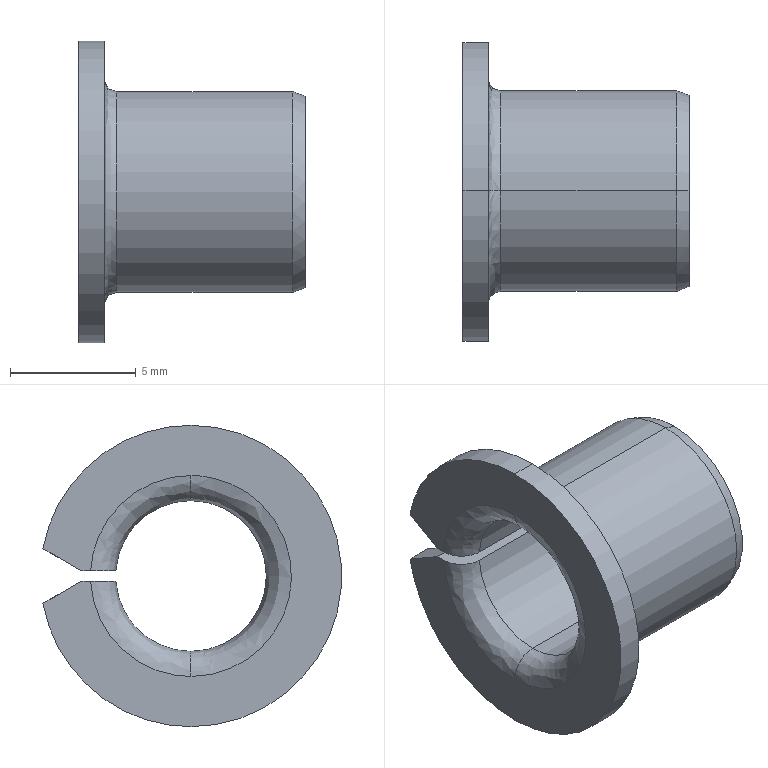Part | SolidWorks | features BaseBody 1 | 1 solid | 28 faces | box 9 x 11.899 x 12 mm | volume 248.45 mm3 | cylinder 9 | plane 7 | spline 6 | cone 6 | commonest cylinder face diameters 6 x3 8 x3 12 x3
STEP:
#1=CARTESIAN_POINT('',(1.5,0.,-4.));
#2=VERTEX_POINT('',#1);
#3=CARTESIAN_POINT('',(1.5,3.995,-0.2));
#4=VERTEX_POINT('',#3);
#5=CARTESIAN_POINT('',(1.5,0.,0.));
#6=DIRECTION('',(1.,0.,0.));
#7=DIRECTION('',(0.,0.,-1.));
#8=AXIS2_PLACEMENT_3D('',#5,#6,#7);
#9=CIRCLE('',#8,4.);
#10=EDGE_CURVE('',#2,#4,#9,.T.);
#11=ORIENTED_EDGE('',*,*,#10,.F.);
#12=CARTESIAN_POINT('',(1.,-0.000000039,-4.5));
#13=VERTEX_POINT('',#12);
#14=CARTESIAN_POINT('',(1.5,0.,-4.5));
#15=DIRECTION('',(0.,-1.,0.));
#16=DIRECTION('',(0.,0.,-1.));
#17=AXIS2_PLACEMENT_3D('',#14,#15,#16);
#18=CIRCLE('',#17,0.5);
#19=EDGE_CURVE('',#2,#13,#18,.T.);
#20=ORIENTED_EDGE('',*,*,#19,.T.);
#21=CARTESIAN_POINT('',(1.,4.491,-0.2835));
#22=VERTEX_POINT('',#21);
#23=CARTESIAN_POINT('',(1.,4.491,-0.2835));
#24=CARTESIAN_POINT('',(1.,4.456,-0.8322));
#25=CARTESIAN_POINT('',(1.,4.326,-1.356));
#26=CARTESIAN_POINT('',(1.,4.071,-1.919));
#27=CARTESIAN_POINT('',(1.,4.039,-1.986));
#28=CARTESIAN_POINT('',(1.,3.973,-2.115));
#29=CARTESIAN_POINT('',(1.,3.869,-2.306));
#30=CARTESIAN_POINT('',(1.,3.751,-2.49));
#31=CARTESIAN_POINT('',(1.,3.582,-2.727));
#32=CARTESIAN_POINT('',(1.,3.49,-2.845));
#33=CARTESIAN_POINT('',(1.,3.295,-3.068));
#34=CARTESIAN_POINT('',(1.,3.193,-3.175));
#35=CARTESIAN_POINT('',(1.,2.868,-3.48));
#36=CARTESIAN_POINT('',(1.,2.633,-3.661));
#37=CARTESIAN_POINT('',(1.,2.255,-3.897));
#38=CARTESIAN_POINT('',(1.,2.129,-3.967));
#39=CARTESIAN_POINT('',(1.,1.869,-4.096));
#40=CARTESIAN_POINT('',(1.,1.703,-4.169));
#41=CARTESIAN_POINT('',(1.,1.532,-4.231));
#42=CARTESIAN_POINT('',(1.,1.464,-4.256));
#43=CARTESIAN_POINT('',(1.,1.433,-4.266));
#44=CARTESIAN_POINT('',(1.,1.335,-4.298));
#45=CARTESIAN_POINT('',(1.,1.14,-4.357));
#46=CARTESIAN_POINT('',(1.,0.678,-4.464));
#47=CARTESIAN_POINT('',(1.,0.2735,-4.5));
#48=CARTESIAN_POINT('',(1.,-0.000000039,-4.5));
#49=B_SPLINE_CURVE_WITH_KNOTS('',3,(#23,#24,#25,#26,#27,#28,#29,#30,#31,#32,#33,#34,#35,#36,#37,#38,#39,#40,#41,#42,#43,#44,#45,#46,#47,#48),.UNSPECIFIED.,.F.,.F.,(4,2,2,1,2,2,2,2,2,1,2,2,1,1,4),(0.,0.06118,0.06883,0.07648,0.09177,0.1071,0.1224,0.153,0.1682,0.1835,0.1874,0.1912,0.1988,0.2141,0.2447),.UNSPECIFIED.);
#50=EDGE_CURVE('',#22,#13,#49,.T.);
#51=ORIENTED_EDGE('',*,*,#50,.F.);
#52=CARTESIAN_POINT('',(1.023,4.346,-0.2));
#53=VERTEX_POINT('',#52);
#54=CARTESIAN_POINT('',(1.,4.491,-0.2835));
#55=CARTESIAN_POINT('',(1.,4.442,-0.2552));
#56=CARTESIAN_POINT('',(1.008,4.394,-0.2273));
#57=CARTESIAN_POINT('',(1.023,4.346,-0.2));
#58=B_SPLINE_CURVE_WITH_KNOTS('',3,(#54,#55,#56,#57),.UNSPECIFIED.,.F.,.F.,(4,4),(0.,0.0001686),.UNSPECIFIED.);
#59=EDGE_CURVE('',#22,#53,#58,.T.);
#60=ORIENTED_EDGE('',*,*,#59,.T.);
#61=CARTESIAN_POINT('',(1.023,4.346,-0.2));
#62=CARTESIAN_POINT('',(1.054,4.245,-0.2));
#63=CARTESIAN_POINT('',(1.118,4.156,-0.2));
#64=CARTESIAN_POINT('',(1.289,4.03,-0.2));
#65=CARTESIAN_POINT('',(1.393,3.995,-0.2));
#66=CARTESIAN_POINT('',(1.5,3.995,-0.2));
#67=B_SPLINE_CURVE_WITH_KNOTS('',3,(#61,#62,#63,#64,#65,#66),.UNSPECIFIED.,.F.,.F.,(4,2,4),(0.,0.0003154,0.0006309),.UNSPECIFIED.);
#68=EDGE_CURVE('',#53,#4,#67,.T.);
#69=ORIENTED_EDGE('',*,*,#68,.T.);
#70=EDGE_LOOP('',(#11,#20,#51,#60,#69));
#71=FACE_OUTER_BOUND('',#70,.T.);
#72=CARTESIAN_POINT('',(1.5,3.997,-0.1473));
#73=CARTESIAN_POINT('',(1.5,3.913,-2.421));
#74=CARTESIAN_POINT('',(1.5,2.275,-4.));
#75=CARTESIAN_POINT('',(1.5,-0.000000035,-4.));
#76=CARTESIAN_POINT('',(1.207,3.997,-0.1473));
#77=CARTESIAN_POINT('',(1.207,3.913,-2.421));
#78=CARTESIAN_POINT('',(1.207,2.275,-4.));
#79=CARTESIAN_POINT('',(1.207,-0.000000035,-4.));
#80=CARTESIAN_POINT('',(1.,4.204,-0.1549));
#81=CARTESIAN_POINT('',(1.,4.116,-2.546));
#82=CARTESIAN_POINT('',(1.,2.393,-4.207));
#83=CARTESIAN_POINT('',(1.,-0.000000037,-4.207));
#84=CARTESIAN_POINT('',(1.,4.497,-0.1657));
#85=CARTESIAN_POINT('',(1.,4.403,-2.724));
#86=CARTESIAN_POINT('',(1.,2.56,-4.5));
#87=CARTESIAN_POINT('',(1.,-0.000000039,-4.5));
#88=(BOUNDED_SURFACE()B_SPLINE_SURFACE(3,3,((#72,#73,#74,#75),(#76,#77,#78,#79),(#80,#81,#82,#83),(#84,#85,#86,#87)),.UNSPECIFIED.,.F.,.F.,.F.)B_SPLINE_SURFACE_WITH_KNOTS((4,4),(4,4),(0.,1.),(0.,1.),.UNSPECIFIED.)GEOMETRIC_REPRESENTATION_ITEM()RATIONAL_B_SPLINE_SURFACE(((1.,0.8133,0.8133,1.),(0.8047,0.6545,0.6545,0.8047),(0.8047,0.6545,0.6545,0.8047),(1.,0.8133,0.8133,1.)))REPRESENTATION_ITEM('')SURFACE());
#89=ADVANCED_FACE('',(#71),#88,.F.);
#90=ORIENTED_EDGE('',*,*,#19,.F.);
#91=CARTESIAN_POINT('',(1.5,0.,4.));
#92=VERTEX_POINT('',#91);
#93=CARTESIAN_POINT('',(1.5,0.,0.));
#94=DIRECTION('',(1.,0.,0.));
#95=DIRECTION('',(0.,0.,-1.));
#96=AXIS2_PLACEMENT_3D('',#93,#94,#95);
#97=CIRCLE('',#96,4.);
#98=EDGE_CURVE('',#92,#2,#97,.T.);
#99=ORIENTED_EDGE('',*,*,#98,.F.);
#100=CARTESIAN_POINT('',(1.,-0.000000067,4.5));
#101=VERTEX_POINT('',#100);
#102=CARTESIAN_POINT('',(1.5,0.,4.5));
#103=DIRECTION('',(0.,1.,0.));
#104=DIRECTION('',(0.,0.,1.));
#105=AXIS2_PLACEMENT_3D('',#102,#103,#104);
#106=CIRCLE('',#105,0.5);
#107=EDGE_CURVE('',#92,#101,#106,.T.);
#108=ORIENTED_EDGE('',*,*,#107,.T.);
#109=CARTESIAN_POINT('',(1.,-0.000000039,-4.5));
#110=CARTESIAN_POINT('',(1.,-0.2853,-4.5));
#111=CARTESIAN_POINT('',(1.,-0.5701,-4.473));
#112=CARTESIAN_POINT('',(1.,-1.124,-4.367));
#113=CARTESIAN_POINT('',(1.,-1.395,-4.288));
#114=CARTESIAN_POINT('',(1.,-1.793,-4.13));
#115=CARTESIAN_POINT('',(1.,-1.934,-4.066));
#116=CARTESIAN_POINT('',(1.,-2.202,-3.927));
#117=CARTESIAN_POINT('',(1.,-2.333,-3.851));
#118=CARTESIAN_POINT('',(1.,-2.587,-3.685));
#119=CARTESIAN_POINT('',(1.,-2.713,-3.593));
#120=CARTESIAN_POINT('',(1.,-2.953,-3.399));
#121=CARTESIAN_POINT('',(1.,-3.068,-3.296));
#122=CARTESIAN_POINT('',(1.,-3.397,-2.967));
#123=CARTESIAN_POINT('',(1.,-3.592,-2.728));
#124=CARTESIAN_POINT('',(1.,-3.848,-2.339));
#125=CARTESIAN_POINT('',(1.,-3.923,-2.21));
#126=CARTESIAN_POINT('',(1.,-4.063,-1.941));
#127=CARTESIAN_POINT('',(1.,-4.125,-1.804));
#128=CARTESIAN_POINT('',(1.,-4.21,-1.592));
#129=CARTESIAN_POINT('',(1.,-4.234,-1.527));
#130=CARTESIAN_POINT('',(1.,-4.28,-1.392));
#131=CARTESIAN_POINT('',(1.,-4.345,-1.189));
#132=CARTESIAN_POINT('',(1.,-4.394,-0.9837));
#133=CARTESIAN_POINT('',(1.,-4.473,-0.5685));
#134=CARTESIAN_POINT('',(1.,-4.5,-0.2864));
#135=CARTESIAN_POINT('',(1.,-4.5,0.2866));
#136=CARTESIAN_POINT('',(1.,-4.46,0.709));
#137=CARTESIAN_POINT('',(1.,-4.345,1.189));
#138=CARTESIAN_POINT('',(1.,-4.28,1.392));
#139=CARTESIAN_POINT('',(1.,-4.234,1.527));
#140=CARTESIAN_POINT('',(1.,-4.21,1.592));
#141=CARTESIAN_POINT('',(1.,-4.126,1.803));
#142=CARTESIAN_POINT('',(1.,-4.063,1.941));
#143=CARTESIAN_POINT('',(1.,-3.923,2.209));
#144=CARTESIAN_POINT('',(1.,-3.847,2.339));
#145=CARTESIAN_POINT('',(1.,-3.593,2.727));
#146=CARTESIAN_POINT('',(1.,-3.397,2.968));
#147=CARTESIAN_POINT('',(1.,-3.068,3.295));
#148=CARTESIAN_POINT('',(1.,-2.954,3.399));
#149=CARTESIAN_POINT('',(1.,-2.714,3.593));
#150=CARTESIAN_POINT('',(1.,-2.587,3.685));
#151=CARTESIAN_POINT('',(1.,-2.333,3.851));
#152=CARTESIAN_POINT('',(1.,-2.203,3.927));
#153=CARTESIAN_POINT('',(1.,-1.934,4.066));
#154=CARTESIAN_POINT('',(1.,-1.793,4.13));
#155=CARTESIAN_POINT('',(1.,-1.395,4.288));
#156=CARTESIAN_POINT('',(1.,-1.124,4.367));
#157=CARTESIAN_POINT('',(1.,-0.5704,4.473));
#158=CARTESIAN_POINT('',(1.,-0.285,4.5));
#159=CARTESIAN_POINT('',(1.,-0.000000067,4.5));
#160=B_SPLINE_CURVE_WITH_KNOTS('',3,(#109,#110,#111,#112,#113,#114,#115,#116,#117,#118,#119,#120,#121,#122,#123,#124,#125,#126,#127,#128,#129,#130,#131,#132,#133,#134,#135,#136,#137,#138,#139,#140,#141,#142,#143,#144,#145,#146,#147,#148,#149,#150,#151,#152,#153,#154,#155,#156,#157,#158,#159),.UNSPECIFIED.,.F.,.F.,(4,2,2,2,2,2,2,2,2,2,2,1,2,2,1,1,2,2,2,2,2,2,2,2,2,2,4),(0.2447,0.2766,0.3085,0.3245,0.3405,0.3564,0.3724,0.4043,0.4202,0.4362,0.4442,0.4521,0.4681,0.5,0.5319,0.5479,0.5558,0.5638,0.5798,0.5957,0.6276,0.6436,0.6596,0.6755,0.6915,0.7234,0.7553),.UNSPECIFIED.);
#161=EDGE_CURVE('',#13,#101,#160,.T.);
#162=ORIENTED_EDGE('',*,*,#161,.F.);
#163=EDGE_LOOP('',(#90,#99,#108,#162));
#164=FACE_OUTER_BOUND('',#163,.T.);
#165=CARTESIAN_POINT('',(1.5,0.,-4.));
#166=CARTESIAN_POINT('',(1.5,-8.,-4.));
#167=CARTESIAN_POINT('',(1.5,-8.,4.));
#168=CARTESIAN_POINT('',(1.5,0.,4.));
#169=CARTESIAN_POINT('',(1.207,0.,-4.));
#170=CARTESIAN_POINT('',(1.207,-8.,-4.));
#171=CARTESIAN_POINT('',(1.207,-8.,4.));
#172=CARTESIAN_POINT('',(1.207,0.,4.));
#173=CARTESIAN_POINT('',(1.,0.,-4.207));
#174=CARTESIAN_POINT('',(1.,-8.414,-4.207));
#175=CARTESIAN_POINT('',(1.,-8.414,4.207));
#176=CARTESIAN_POINT('',(1.,0.,4.207));
#177=CARTESIAN_POINT('',(1.,0.,-4.5));
#178=CARTESIAN_POINT('',(1.,-9.,-4.5));
#179=CARTESIAN_POINT('',(1.,-9.,4.5));
#180=CARTESIAN_POINT('',(1.,0.,4.5));
#181=(BOUNDED_SURFACE()B_SPLINE_SURFACE(3,3,((#165,#166,#167,#168),(#169,#170,#171,#172),(#173,#174,#175,#176),(#177,#178,#179,#180)),.UNSPECIFIED.,.F.,.F.,.T.)B_SPLINE_SURFACE_WITH_KNOTS((4,4),(4,4),(0.,1.),(0.,1.),.UNSPECIFIED.)GEOMETRIC_REPRESENTATION_ITEM()RATIONAL_B_SPLINE_SURFACE(((1.,0.3333,0.3333,1.),(0.8047,0.2682,0.2682,0.8047),(0.8047,0.2682,0.2682,0.8047),(1.,0.3333,0.3333,1.)))REPRESENTATION_ITEM('')SURFACE());
#182=ADVANCED_FACE('',(#164),#181,.F.);
#183=CARTESIAN_POINT('',(1.,0.,3.));
#184=VERTEX_POINT('',#183);
#185=CARTESIAN_POINT('',(1.,0.,-3.));
#186=VERTEX_POINT('',#185);
#187=CARTESIAN_POINT('',(1.,0.,0.));
#188=DIRECTION('',(1.,0.,0.));
#189=DIRECTION('',(0.,0.,-1.));
#190=AXIS2_PLACEMENT_3D('',#187,#188,#189);
#191=CIRCLE('',#190,3.);
#192=EDGE_CURVE('',#184,#186,#191,.T.);
#193=ORIENTED_EDGE('',*,*,#192,.T.);
#194=CARTESIAN_POINT('',(0.,-0.000000037,-4.));
#195=VERTEX_POINT('',#194);
#196=CARTESIAN_POINT('',(1.,0.,-4.));
#197=DIRECTION('',(0.,-1.,0.));
#198=DIRECTION('',(0.,0.,-1.));
#199=AXIS2_PLACEMENT_3D('',#196,#197,#198);
#200=CIRCLE('',#199,1.);
#201=EDGE_CURVE('',#186,#195,#200,.T.);
#202=ORIENTED_EDGE('',*,*,#201,.T.);
#203=CARTESIAN_POINT('',(0.,-0.000000017,4.));
#204=VERTEX_POINT('',#203);
#205=CARTESIAN_POINT('',(0.,-0.000000037,-4.));
#206=CARTESIAN_POINT('',(0.,-8.,-4.));
#207=CARTESIAN_POINT('',(0.,-8.,4.));
#208=CARTESIAN_POINT('',(0.,-0.000000017,4.));
#209=(BOUNDED_CURVE()B_SPLINE_CURVE(3,(#205,#206,#207,#208),.UNSPECIFIED.,.F.,.F.)B_SPLINE_CURVE_WITH_KNOTS((4,4),(0.246,0.754),.UNSPECIFIED.)CURVE()GEOMETRIC_REPRESENTATION_ITEM()RATIONAL_B_SPLINE_CURVE((1.,0.3333,0.3333,1.))REPRESENTATION_ITEM(''));
#210=EDGE_CURVE('',#195,#204,#209,.T.);
#211=ORIENTED_EDGE('',*,*,#210,.T.);
#212=CARTESIAN_POINT('',(1.,0.,4.));
#213=DIRECTION('',(0.,1.,0.));
#214=DIRECTION('',(0.,0.,1.));
#215=AXIS2_PLACEMENT_3D('',#212,#213,#214);
#216=CIRCLE('',#215,1.);
#217=EDGE_CURVE('',#184,#204,#216,.T.);
#218=ORIENTED_EDGE('',*,*,#217,.F.);
#219=EDGE_LOOP('',(#193,#202,#211,#218));
#220=FACE_OUTER_BOUND('',#219,.T.);
#221=CARTESIAN_POINT('',(1.,0.,-3.));
#222=CARTESIAN_POINT('',(1.,-6.,-3.));
#223=CARTESIAN_POINT('',(1.,-6.,3.));
#224=CARTESIAN_POINT('',(1.,0.,3.));
#225=CARTESIAN_POINT('',(0.4142,0.,-3.));
#226=CARTESIAN_POINT('',(0.4142,-6.,-3.));
#227=CARTESIAN_POINT('',(0.4142,-6.,3.));
#228=CARTESIAN_POINT('',(0.4142,0.,3.));
#229=CARTESIAN_POINT('',(0.,0.,-3.414));
#230=CARTESIAN_POINT('',(0.,-6.828,-3.414));
#231=CARTESIAN_POINT('',(0.,-6.828,3.414));
#232=CARTESIAN_POINT('',(0.,0.,3.414));
#233=CARTESIAN_POINT('',(0.,0.,-4.));
#234=CARTESIAN_POINT('',(0.,-8.,-4.));
#235=CARTESIAN_POINT('',(0.,-8.,4.));
#236=CARTESIAN_POINT('',(0.,0.,4.));
#237=(BOUNDED_SURFACE()B_SPLINE_SURFACE(3,3,((#221,#222,#223,#224),(#225,#226,#227,#228),(#229,#230,#231,#232),(#233,#234,#235,#236)),.UNSPECIFIED.,.F.,.F.,.T.)B_SPLINE_SURFACE_WITH_KNOTS((4,4),(4,4),(0.,1.),(0.,1.),.UNSPECIFIED.)GEOMETRIC_REPRESENTATION_ITEM()RATIONAL_B_SPLINE_SURFACE(((1.,0.3333,0.3333,1.),(0.8047,0.2682,0.2682,0.8047),(0.8047,0.2682,0.2682,0.8047),(1.,0.3333,0.3333,1.)))REPRESENTATION_ITEM('')SURFACE());
#238=ADVANCED_FACE('',(#220),#237,.T.);
#239=CARTESIAN_POINT('',(1.,2.993,0.2));
#240=VERTEX_POINT('',#239);
#241=CARTESIAN_POINT('',(1.,0.,0.));
#242=DIRECTION('',(1.,0.,0.));
#243=DIRECTION('',(0.,0.,-1.));
#244=AXIS2_PLACEMENT_3D('',#241,#242,#243);
#245=CIRCLE('',#244,3.);
#246=EDGE_CURVE('',#240,#184,#245,.T.);
#247=ORIENTED_EDGE('',*,*,#246,.T.);
#248=ORIENTED_EDGE('',*,*,#217,.T.);
#249=CARTESIAN_POINT('',(0.,3.995,0.2));
#250=VERTEX_POINT('',#249);
#251=CARTESIAN_POINT('',(0.,-0.000000017,4.));
#252=CARTESIAN_POINT('',(0.,2.251,4.));
#253=CARTESIAN_POINT('',(0.,3.882,2.448));
#254=CARTESIAN_POINT('',(0.,3.995,0.2));
#255=(BOUNDED_CURVE()B_SPLINE_CURVE(3,(#251,#252,#253,#254),.UNSPECIFIED.,.F.,.F.)B_SPLINE_CURVE_WITH_KNOTS((4,4),(0.754,1.),.UNSPECIFIED.)CURVE()GEOMETRIC_REPRESENTATION_ITEM()RATIONAL_B_SPLINE_CURVE((1.,0.8164,0.8164,1.))REPRESENTATION_ITEM(''));
#256=EDGE_CURVE('',#204,#250,#255,.T.);
#257=ORIENTED_EDGE('',*,*,#256,.T.);
#258=CARTESIAN_POINT('',(0.,3.995,0.2));
#259=CARTESIAN_POINT('',(0.,3.863,0.2));
#260=CARTESIAN_POINT('',(0.02595,3.733,0.2));
#261=CARTESIAN_POINT('',(0.1261,3.491,0.2));
#262=CARTESIAN_POINT('',(0.2003,3.38,0.2));
#263=CARTESIAN_POINT('',(0.4767,3.102,0.2));
#264=CARTESIAN_POINT('',(0.7357,2.993,0.2));
#265=CARTESIAN_POINT('',(1.,2.993,0.2));
#266=B_SPLINE_CURVE_WITH_KNOTS('',3,(#258,#259,#260,#261,#262,#263,#264,#265),.UNSPECIFIED.,.F.,.F.,(4,2,2,4),(0.,0.0003909,0.0007817,0.001563),.UNSPECIFIED.);
#267=EDGE_CURVE('',#250,#240,#266,.T.);
#268=ORIENTED_EDGE('',*,*,#267,.T.);
#269=EDGE_LOOP('',(#247,#248,#257,#268));
#270=FACE_OUTER_BOUND('',#269,.T.);
#271=CARTESIAN_POINT('',(1.,-0.000000006,3.));
#272=CARTESIAN_POINT('',(1.,1.701,3.));
#273=CARTESIAN_POINT('',(1.,2.928,1.822));
#274=CARTESIAN_POINT('',(1.,2.997,0.1227));
#275=CARTESIAN_POINT('',(0.4142,-0.000000006,3.));
#276=CARTESIAN_POINT('',(0.4142,1.701,3.));
#277=CARTESIAN_POINT('',(0.4142,2.928,1.822));
#278=CARTESIAN_POINT('',(0.4142,2.997,0.1227));
#279=CARTESIAN_POINT('',(0.,-0.000000007,3.414));
#280=CARTESIAN_POINT('',(0.,1.936,3.414));
#281=CARTESIAN_POINT('',(0.,3.332,2.074));
#282=CARTESIAN_POINT('',(0.,3.411,0.1396));
#283=CARTESIAN_POINT('',(0.,-0.000000008,4.));
#284=CARTESIAN_POINT('',(0.,2.268,4.));
#285=CARTESIAN_POINT('',(0.,3.904,2.43));
#286=CARTESIAN_POINT('',(0.,3.997,0.1635));
#287=(BOUNDED_SURFACE()B_SPLINE_SURFACE(3,3,((#271,#272,#273,#274),(#275,#276,#277,#278),(#279,#280,#281,#282),(#283,#284,#285,#286)),.UNSPECIFIED.,.F.,.F.,.F.)B_SPLINE_SURFACE_WITH_KNOTS((4,4),(4,4),(0.,1.),(0.,1.),.UNSPECIFIED.)GEOMETRIC_REPRESENTATION_ITEM()RATIONAL_B_SPLINE_SURFACE(((1.,0.8143,0.8143,1.),(0.8047,0.6553,0.6553,0.8047),(0.8047,0.6553,0.6553,0.8047),(1.,0.8143,0.8143,1.)))REPRESENTATION_ITEM('')SURFACE());
#288=ADVANCED_FACE('',(#270),#287,.T.);
#289=CARTESIAN_POINT('',(1.5,3.995,0.2));
#290=VERTEX_POINT('',#289);
#291=CARTESIAN_POINT('',(1.5,0.,0.));
#292=DIRECTION('',(1.,0.,0.));
#293=DIRECTION('',(0.,0.,-1.));
#294=AXIS2_PLACEMENT_3D('',#291,#292,#293);
#295=CIRCLE('',#294,4.);
#296=EDGE_CURVE('',#290,#92,#295,.T.);
#297=ORIENTED_EDGE('',*,*,#296,.T.);
#298=CARTESIAN_POINT('',(8.5,0.,4.));
#299=VERTEX_POINT('',#298);
#300=CARTESIAN_POINT('',(5.,0.,4.));
#301=DIRECTION('',(1.,0.,0.));
#302=VECTOR('',#301,1000.);
#303=LINE('',#300,#302);
#304=EDGE_CURVE('',#92,#299,#303,.T.);
#305=ORIENTED_EDGE('',*,*,#304,.T.);
#306=CARTESIAN_POINT('',(8.5,3.995,0.2));
#307=VERTEX_POINT('',#306);
#308=CARTESIAN_POINT('',(8.5,0.,0.));
#309=DIRECTION('',(-1.,0.,0.));
#310=DIRECTION('',(0.,0.,-1.));
#311=AXIS2_PLACEMENT_3D('',#308,#309,#310);
#312=CIRCLE('',#311,4.);
#313=EDGE_CURVE('',#299,#307,#312,.T.);
#314=ORIENTED_EDGE('',*,*,#313,.T.);
#315=CARTESIAN_POINT('',(5.,3.995,0.2));
#316=DIRECTION('',(-1.,0.,0.));
#317=VECTOR('',#316,1000.);
#318=LINE('',#315,#317);
#319=EDGE_CURVE('',#307,#290,#318,.T.);
#320=ORIENTED_EDGE('',*,*,#319,.T.);
#321=EDGE_LOOP('',(#297,#305,#314,#320));
#322=FACE_OUTER_BOUND('',#321,.T.);
#323=CARTESIAN_POINT('',(5.,0.,0.));
#324=DIRECTION('',(1.,0.,0.));
#325=DIRECTION('',(0.,0.,-1.));
#326=AXIS2_PLACEMENT_3D('',#323,#324,#325);
#327=CYLINDRICAL_SURFACE('',#326,4.);
#328=ADVANCED_FACE('',(#322),#327,.T.);
#329=ORIENTED_EDGE('',*,*,#304,.F.);
#330=ORIENTED_EDGE('',*,*,#98,.T.);
#331=CARTESIAN_POINT('',(8.5,0.,-4.));
#332=VERTEX_POINT('',#331);
#333=CARTESIAN_POINT('',(5.,0.,-4.));
#334=DIRECTION('',(1.,0.,0.));
#335=VECTOR('',#334,1000.);
#336=LINE('',#333,#335);
#337=EDGE_CURVE('',#2,#332,#336,.T.);
#338=ORIENTED_EDGE('',*,*,#337,.T.);
#339=CARTESIAN_POINT('',(8.5,0.,0.));
#340=DIRECTION('',(-1.,0.,0.));
#341=DIRECTION('',(0.,0.,-1.));
#342=AXIS2_PLACEMENT_3D('',#339,#340,#341);
#343=CIRCLE('',#342,4.);
#344=EDGE_CURVE('',#332,#299,#343,.T.);
#345=ORIENTED_EDGE('',*,*,#344,.T.);
#346=EDGE_LOOP('',(#329,#330,#338,#345));
#347=FACE_OUTER_BOUND('',#346,.T.);
#348=CARTESIAN_POINT('',(5.,0.,0.));
#349=DIRECTION('',(1.,0.,0.));
#350=DIRECTION('',(0.,0.,-1.));
#351=AXIS2_PLACEMENT_3D('',#348,#349,#350);
#352=CYLINDRICAL_SURFACE('',#351,4.);
#353=ADVANCED_FACE('',(#347),#352,.T.);
#354=CARTESIAN_POINT('',(9.,3.813,-0.2));
#355=VERTEX_POINT('',#354);
#356=CARTESIAN_POINT('',(9.,0.,-3.818));
#357=VERTEX_POINT('',#356);
#358=CARTESIAN_POINT('',(9.,0.,0.));
#359=DIRECTION('',(-1.,0.,0.));
#360=DIRECTION('',(0.,0.,1.));
#361=AXIS2_PLACEMENT_3D('',#358,#359,#360);
#362=CIRCLE('',#361,3.818);
#363=EDGE_CURVE('',#355,#357,#362,.T.);
#364=ORIENTED_EDGE('',*,*,#363,.T.);
#365=CARTESIAN_POINT('',(8.5,0.,-4.));
#366=DIRECTION('',(-0.9397,0.,-0.342));
#367=VECTOR('',#366,1000.);
#368=LINE('',#365,#367);
#369=EDGE_CURVE('',#357,#332,#368,.T.);
#370=ORIENTED_EDGE('',*,*,#369,.T.);
#371=CARTESIAN_POINT('',(8.5,3.995,-0.2));
#372=VERTEX_POINT('',#371);
#373=CARTESIAN_POINT('',(8.5,0.,0.));
#374=DIRECTION('',(-1.,0.,0.));
#375=DIRECTION('',(0.,0.,-1.));
#376=AXIS2_PLACEMENT_3D('',#373,#374,#375);
#377=CIRCLE('',#376,4.);
#378=EDGE_CURVE('',#372,#332,#377,.T.);
#379=ORIENTED_EDGE('',*,*,#378,.F.);
#380=CARTESIAN_POINT('',(8.5,3.995,-0.2));
#381=CARTESIAN_POINT('',(8.667,3.934,-0.2));
#382=CARTESIAN_POINT('',(8.833,3.874,-0.2));
#383=CARTESIAN_POINT('',(9.,3.813,-0.2));
#384=B_SPLINE_CURVE_WITH_KNOTS('',3,(#380,#381,#382,#383),.UNSPECIFIED.,.F.,.F.,(4,4),(0.,0.0005322),.UNSPECIFIED.);
#385=EDGE_CURVE('',#372,#355,#384,.T.);
#386=ORIENTED_EDGE('',*,*,#385,.T.);
#387=EDGE_LOOP('',(#364,#370,#379,#386));
#388=FACE_OUTER_BOUND('',#387,.T.);
#389=CARTESIAN_POINT('',(8.5,0.,0.));
#390=DIRECTION('',(-1.,0.,0.));
#391=DIRECTION('',(0.,0.,1.));
#392=AXIS2_PLACEMENT_3D('',#389,#390,#391);
#393=CONICAL_SURFACE('',#392,4.,0.3491);
#394=ADVANCED_FACE('',(#388),#393,.T.);
#395=ORIENTED_EDGE('',*,*,#369,.F.);
#396=CARTESIAN_POINT('',(9.,0.,3.818));
#397=VERTEX_POINT('',#396);
#398=CARTESIAN_POINT('',(9.,0.,0.));
#399=DIRECTION('',(-1.,0.,0.));
#400=DIRECTION('',(0.,0.,1.));
#401=AXIS2_PLACEMENT_3D('',#398,#399,#400);
#402=CIRCLE('',#401,3.818);
#403=EDGE_CURVE('',#357,#397,#402,.T.);
#404=ORIENTED_EDGE('',*,*,#403,.T.);
#405=CARTESIAN_POINT('',(8.5,0.,4.));
#406=DIRECTION('',(-0.9397,0.,0.342));
#407=VECTOR('',#406,1000.);
#408=LINE('',#405,#407);
#409=EDGE_CURVE('',#397,#299,#408,.T.);
#410=ORIENTED_EDGE('',*,*,#409,.T.);
#411=ORIENTED_EDGE('',*,*,#344,.F.);
#412=EDGE_LOOP('',(#395,#404,#410,#411));
#413=FACE_OUTER_BOUND('',#412,.T.);
#414=CARTESIAN_POINT('',(8.5,0.,0.));
#415=DIRECTION('',(-1.,0.,0.));
#416=DIRECTION('',(0.,0.,1.));
#417=AXIS2_PLACEMENT_3D('',#414,#415,#416);
#418=CONICAL_SURFACE('',#417,4.,0.3491);
#419=ADVANCED_FACE('',(#413),#418,.T.);
#420=ORIENTED_EDGE('',*,*,#192,.F.);
#421=CARTESIAN_POINT('',(8.5,0.,3.));
#422=VERTEX_POINT('',#421);
#423=CARTESIAN_POINT('',(4.75,0.,3.));
#424=DIRECTION('',(1.,0.,0.));
#425=VECTOR('',#424,1000.);
#426=LINE('',#423,#425);
#427=EDGE_CURVE('',#184,#422,#426,.T.);
#428=ORIENTED_EDGE('',*,*,#427,.T.);
#429=CARTESIAN_POINT('',(8.5,0.,-3.));
#430=VERTEX_POINT('',#429);
#431=CARTESIAN_POINT('',(8.5,0.,0.));
#432=DIRECTION('',(-1.,0.,0.));
#433=DIRECTION('',(0.,0.,-1.));
#434=AXIS2_PLACEMENT_3D('',#431,#432,#433);
#435=CIRCLE('',#434,3.);
#436=EDGE_CURVE('',#430,#422,#435,.T.);
#437=ORIENTED_EDGE('',*,*,#436,.F.);
#438=CARTESIAN_POINT('',(4.75,0.,-3.));
#439=DIRECTION('',(1.,0.,0.));
#440=VECTOR('',#439,1000.);
#441=LINE('',#438,#440);
#442=EDGE_CURVE('',#186,#430,#441,.T.);
#443=ORIENTED_EDGE('',*,*,#442,.F.);
#444=EDGE_LOOP('',(#420,#428,#437,#443));
#445=FACE_OUTER_BOUND('',#444,.T.);
#446=CARTESIAN_POINT('',(4.75,0.,0.));
#447=DIRECTION('',(1.,0.,0.));
#448=DIRECTION('',(0.,0.,-1.));
#449=AXIS2_PLACEMENT_3D('',#446,#447,#448);
#450=CYLINDRICAL_SURFACE('',#449,3.);
#451=ADVANCED_FACE('',(#445),#450,.F.);
#452=CARTESIAN_POINT('',(1.,2.993,-0.2));
#453=VERTEX_POINT('',#452);
#454=CARTESIAN_POINT('',(1.,0.,0.));
#455=DIRECTION('',(1.,0.,0.));
#456=DIRECTION('',(0.,0.,-1.));
#457=AXIS2_PLACEMENT_3D('',#454,#455,#456);
#458=CIRCLE('',#457,3.);
#459=EDGE_CURVE('',#186,#453,#458,.T.);
#460=ORIENTED_EDGE('',*,*,#459,.F.);
#461=ORIENTED_EDGE('',*,*,#442,.T.);
#462=CARTESIAN_POINT('',(8.5,2.993,-0.2));
#463=VERTEX_POINT('',#462);
#464=CARTESIAN_POINT('',(8.5,0.,0.));
#465=DIRECTION('',(-1.,0.,0.));
#466=DIRECTION('',(0.,0.,-1.));
#467=AXIS2_PLACEMENT_3D('',#464,#465,#466);
#468=CIRCLE('',#467,3.);
#469=EDGE_CURVE('',#463,#430,#468,.T.);
#470=ORIENTED_EDGE('',*,*,#469,.F.);
#471=CARTESIAN_POINT('',(0.,2.993,-0.2));
#472=DIRECTION('',(-1.,0.,0.));
#473=VECTOR('',#472,1000.);
#474=LINE('',#471,#473);
#475=EDGE_CURVE('',#463,#453,#474,.T.);
#476=ORIENTED_EDGE('',*,*,#475,.T.);
#477=EDGE_LOOP('',(#460,#461,#470,#476));
#478=FACE_OUTER_BOUND('',#477,.T.);
#479=CARTESIAN_POINT('',(4.75,0.,0.));
#480=DIRECTION('',(1.,0.,0.));
#481=DIRECTION('',(0.,0.,-1.));
#482=AXIS2_PLACEMENT_3D('',#479,#480,#481);
#483=CYLINDRICAL_SURFACE('',#482,3.);
#484=ADVANCED_FACE('',(#478),#483,.F.);
#485=ORIENTED_EDGE('',*,*,#436,.T.);
#486=CARTESIAN_POINT('',(9.,0.,3.5));
#487=VERTEX_POINT('',#486);
#488=CARTESIAN_POINT('',(9.,0.,3.5));
#489=DIRECTION('',(0.7071,0.,0.7071));
#490=VECTOR('',#489,1000.);
#491=LINE('',#488,#490);
#492=EDGE_CURVE('',#422,#487,#491,.T.);
#493=ORIENTED_EDGE('',*,*,#492,.T.);
#494=CARTESIAN_POINT('',(9.,0.,-3.5));
#495=VERTEX_POINT('',#494);
#496=CARTESIAN_POINT('',(9.,0.,0.));
#497=DIRECTION('',(-1.,0.,0.));
#498=DIRECTION('',(0.,0.,-1.));
#499=AXIS2_PLACEMENT_3D('',#496,#497,#498);
#500=CIRCLE('',#499,3.5);
#501=EDGE_CURVE('',#495,#487,#500,.T.);
#502=ORIENTED_EDGE('',*,*,#501,.F.);
#503=CARTESIAN_POINT('',(9.,0.,-3.5));
#504=DIRECTION('',(0.7071,0.,-0.7071));
#505=VECTOR('',#504,1000.);
#506=LINE('',#503,#505);
#507=EDGE_CURVE('',#430,#495,#506,.T.);
#508=ORIENTED_EDGE('',*,*,#507,.F.);
#509=EDGE_LOOP('',(#485,#493,#502,#508));
#510=FACE_OUTER_BOUND('',#509,.T.);
#511=CARTESIAN_POINT('',(9.,0.,0.));
#512=DIRECTION('',(1.,0.,0.));
#513=DIRECTION('',(0.,0.,-1.));
#514=AXIS2_PLACEMENT_3D('',#511,#512,#513);
#515=CONICAL_SURFACE('',#514,3.5,0.7854);
#516=ADVANCED_FACE('',(#510),#515,.F.);
#517=ORIENTED_EDGE('',*,*,#469,.T.);
#518=ORIENTED_EDGE('',*,*,#507,.T.);
#519=CARTESIAN_POINT('',(9.,3.494,-0.2));
#520=VERTEX_POINT('',#519);
#521=CARTESIAN_POINT('',(9.,0.,0.));
#522=DIRECTION('',(-1.,0.,0.));
#523=DIRECTION('',(0.,0.,-1.));
#524=AXIS2_PLACEMENT_3D('',#521,#522,#523);
#525=CIRCLE('',#524,3.5);
#526=EDGE_CURVE('',#520,#495,#525,.T.);
#527=ORIENTED_EDGE('',*,*,#526,.F.);
#528=CARTESIAN_POINT('',(8.5,2.993,-0.2));
#529=CARTESIAN_POINT('',(8.667,3.16,-0.2));
#530=CARTESIAN_POINT('',(8.833,3.327,-0.2));
#531=CARTESIAN_POINT('',(9.,3.494,-0.2));
#532=B_SPLINE_CURVE_WITH_KNOTS('',3,(#528,#529,#530,#531),.UNSPECIFIED.,.F.,.F.,(4,4),(0.,0.0007078),.UNSPECIFIED.);
#533=EDGE_CURVE('',#463,#520,#532,.T.);
#534=ORIENTED_EDGE('',*,*,#533,.F.);
#535=EDGE_LOOP('',(#517,#518,#527,#534));
#536=FACE_OUTER_BOUND('',#535,.T.);
#537=CARTESIAN_POINT('',(9.,0.,0.));
#538=DIRECTION('',(1.,0.,0.));
#539=DIRECTION('',(0.,0.,-1.));
#540=AXIS2_PLACEMENT_3D('',#537,#538,#539);
#541=CONICAL_SURFACE('',#540,3.5,0.7854);
#542=ADVANCED_FACE('',(#536),#541,.F.);
#543=CARTESIAN_POINT('',(0.,0.,6.));
#544=VERTEX_POINT('',#543);
#545=CARTESIAN_POINT('',(0.,5.899,1.096));
#546=VERTEX_POINT('',#545);
#547=CARTESIAN_POINT('',(0.,0.,0.));
#548=DIRECTION('',(-1.,0.,0.));
#549=DIRECTION('',(0.,0.,-1.));
#550=AXIS2_PLACEMENT_3D('',#547,#548,#549);
#551=CIRCLE('',#550,6.);
#552=EDGE_CURVE('',#544,#546,#551,.T.);
#553=ORIENTED_EDGE('',*,*,#552,.F.);
#554=CARTESIAN_POINT('',(1.,0.,6.));
#555=VERTEX_POINT('',#554);
#556=CARTESIAN_POINT('',(0.5,0.,6.));
#557=DIRECTION('',(1.,0.,0.));
#558=VECTOR('',#557,1000.);
#559=LINE('',#556,#558);
#560=EDGE_CURVE('',#544,#555,#559,.T.);
#561=ORIENTED_EDGE('',*,*,#560,.T.);
#562=CARTESIAN_POINT('',(1.,5.899,1.096));
#563=VERTEX_POINT('',#562);
#564=CARTESIAN_POINT('',(1.,0.,0.));
#565=DIRECTION('',(1.,0.,0.));
#566=DIRECTION('',(0.,0.,-1.));
#567=AXIS2_PLACEMENT_3D('',#564,#565,#566);
#568=CIRCLE('',#567,6.);
#569=EDGE_CURVE('',#563,#555,#568,.T.);
#570=ORIENTED_EDGE('',*,*,#569,.F.);
#571=CARTESIAN_POINT('',(0.5,5.899,1.096));
#572=DIRECTION('',(-1.,0.,0.));
#573=VECTOR('',#572,1000.);
#574=LINE('',#571,#573);
#575=EDGE_CURVE('',#563,#546,#574,.T.);
#576=ORIENTED_EDGE('',*,*,#575,.T.);
#577=EDGE_LOOP('',(#553,#561,#570,#576));
#578=FACE_OUTER_BOUND('',#577,.T.);
#579=CARTESIAN_POINT('',(0.5,0.,0.));
#580=DIRECTION('',(1.,0.,0.));
#581=DIRECTION('',(0.,0.,-1.));
#582=AXIS2_PLACEMENT_3D('',#579,#580,#581);
#583=CYLINDRICAL_SURFACE('',#582,6.);
#584=ADVANCED_FACE('',(#578),#583,.T.);
#585=ORIENTED_EDGE('',*,*,#560,.F.);
#586=CARTESIAN_POINT('',(0.,0.,-6.));
#587=VERTEX_POINT('',#586);
#588=CARTESIAN_POINT('',(0.,0.,0.));
#589=DIRECTION('',(-1.,0.,0.));
#590=DIRECTION('',(0.,0.,-1.));
#591=AXIS2_PLACEMENT_3D('',#588,#589,#590);
#592=CIRCLE('',#591,6.);
#593=EDGE_CURVE('',#587,#544,#592,.T.);
#594=ORIENTED_EDGE('',*,*,#593,.F.);
#595=CARTESIAN_POINT('',(1.,0.,-6.));
#596=VERTEX_POINT('',#595);
#597=CARTESIAN_POINT('',(0.5,0.,-6.));
#598=DIRECTION('',(1.,0.,0.));
#599=VECTOR('',#598,1000.);
#600=LINE('',#597,#599);
#601=EDGE_CURVE('',#587,#596,#600,.T.);
#602=ORIENTED_EDGE('',*,*,#601,.T.);
#603=CARTESIAN_POINT('',(1.,0.,0.));
#604=DIRECTION('',(1.,0.,0.));
#605=DIRECTION('',(0.,0.,-1.));
#606=AXIS2_PLACEMENT_3D('',#603,#604,#605);
#607=CIRCLE('',#606,6.);
#608=EDGE_CURVE('',#555,#596,#607,.T.);
#609=ORIENTED_EDGE('',*,*,#608,.F.);
#610=EDGE_LOOP('',(#585,#594,#602,#609));
#611=FACE_OUTER_BOUND('',#610,.T.);
#612=CARTESIAN_POINT('',(0.5,0.,0.));
#613=DIRECTION('',(1.,0.,0.));
#614=DIRECTION('',(0.,0.,-1.));
#615=AXIS2_PLACEMENT_3D('',#612,#613,#614);
#616=CYLINDRICAL_SURFACE('',#615,6.);
#617=ADVANCED_FACE('',(#611),#616,.T.);
#618=ORIENTED_EDGE('',*,*,#337,.F.);
#619=ORIENTED_EDGE('',*,*,#10,.T.);
#620=CARTESIAN_POINT('',(5.,3.995,-0.2));
#621=DIRECTION('',(1.,0.,0.));
#622=VECTOR('',#621,1000.);
#623=LINE('',#620,#622);
#624=EDGE_CURVE('',#4,#372,#623,.T.);
#625=ORIENTED_EDGE('',*,*,#624,.T.);
#626=ORIENTED_EDGE('',*,*,#378,.T.);
#627=EDGE_LOOP('',(#618,#619,#625,#626));
#628=FACE_OUTER_BOUND('',#627,.T.);
#629=CARTESIAN_POINT('',(5.,0.,0.));
#630=DIRECTION('',(1.,0.,0.));
#631=DIRECTION('',(0.,0.,-1.));
#632=AXIS2_PLACEMENT_3D('',#629,#630,#631);
#633=CYLINDRICAL_SURFACE('',#632,4.);
#634=ADVANCED_FACE('',(#628),#633,.T.);
#635=ORIENTED_EDGE('',*,*,#319,.F.);
#636=CARTESIAN_POINT('',(9.,3.813,0.2));
#637=VERTEX_POINT('',#636);
#638=CARTESIAN_POINT('',(9.,3.813,0.2));
#639=CARTESIAN_POINT('',(8.833,3.874,0.2));
#640=CARTESIAN_POINT('',(8.667,3.934,0.2));
#641=CARTESIAN_POINT('',(8.5,3.995,0.2));
#642=B_SPLINE_CURVE_WITH_KNOTS('',3,(#638,#639,#640,#641),.UNSPECIFIED.,.F.,.F.,(4,4),(0.,0.0005322),.UNSPECIFIED.);
#643=EDGE_CURVE('',#637,#307,#642,.T.);
#644=ORIENTED_EDGE('',*,*,#643,.F.);
#645=CARTESIAN_POINT('',(9.,3.494,0.2));
#646=VERTEX_POINT('',#645);
#647=CARTESIAN_POINT('',(9.,3.659,0.2));
#648=DIRECTION('',(0.,1.,0.));
#649=VECTOR('',#648,1000.);
#650=LINE('',#647,#649);
#651=EDGE_CURVE('',#646,#637,#650,.T.);
#652=ORIENTED_EDGE('',*,*,#651,.F.);
#653=CARTESIAN_POINT('',(8.5,2.993,0.2));
#654=VERTEX_POINT('',#653);
#655=CARTESIAN_POINT('',(9.,3.494,0.2));
#656=CARTESIAN_POINT('',(8.833,3.327,0.2));
#657=CARTESIAN_POINT('',(8.667,3.16,0.2));
#658=CARTESIAN_POINT('',(8.5,2.993,0.2));
#659=B_SPLINE_CURVE_WITH_KNOTS('',3,(#655,#656,#657,#658),.UNSPECIFIED.,.F.,.F.,(4,4),(0.,0.0007078),.UNSPECIFIED.);
#660=EDGE_CURVE('',#646,#654,#659,.T.);
#661=ORIENTED_EDGE('',*,*,#660,.T.);
#662=CARTESIAN_POINT('',(0.,2.993,0.2));
#663=DIRECTION('',(1.,0.,0.));
#664=VECTOR('',#663,1000.);
#665=LINE('',#662,#664);
#666=EDGE_CURVE('',#240,#654,#665,.T.);
#667=ORIENTED_EDGE('',*,*,#666,.F.);
#668=ORIENTED_EDGE('',*,*,#267,.F.);
#669=CARTESIAN_POINT('',(0.,4.346,0.2));
#670=VERTEX_POINT('',#669);
#671=CARTESIAN_POINT('',(0.,5.,0.2));
#672=DIRECTION('',(0.,-1.,0.));
#673=VECTOR('',#672,1000.);
#674=LINE('',#671,#673);
#675=EDGE_CURVE('',#670,#250,#674,.T.);
#676=ORIENTED_EDGE('',*,*,#675,.F.);
#677=CARTESIAN_POINT('',(1.023,4.346,0.2));
#678=VERTEX_POINT('',#677);
#679=CARTESIAN_POINT('',(0.,4.346,0.2));
#680=DIRECTION('',(1.,0.,0.));
#681=VECTOR('',#680,1000.);
#682=LINE('',#679,#681);
#683=EDGE_CURVE('',#670,#678,#682,.T.);
#684=ORIENTED_EDGE('',*,*,#683,.T.);
#685=CARTESIAN_POINT('',(1.5,3.995,0.2));
#686=CARTESIAN_POINT('',(1.393,3.995,0.2));
#687=CARTESIAN_POINT('',(1.289,4.029,0.2));
#688=CARTESIAN_POINT('',(1.119,4.155,0.2));
#689=CARTESIAN_POINT('',(1.054,4.245,0.2));
#690=CARTESIAN_POINT('',(1.023,4.346,0.2));
#691=B_SPLINE_CURVE_WITH_KNOTS('',3,(#685,#686,#687,#688,#689,#690),.UNSPECIFIED.,.F.,.F.,(4,2,4),(0.,0.0003154,0.0006309),.UNSPECIFIED.);
#692=EDGE_CURVE('',#290,#678,#691,.T.);
#693=ORIENTED_EDGE('',*,*,#692,.F.);
#694=EDGE_LOOP('',(#635,#644,#652,#661,#667,#668,#676,#684,#693));
#695=FACE_OUTER_BOUND('',#694,.T.);
#696=CARTESIAN_POINT('',(0.,0.,0.2));
#697=DIRECTION('',(0.,0.,1.));
#698=DIRECTION('',(1.,0.,0.));
#699=AXIS2_PLACEMENT_3D('',#696,#697,#698);
#700=PLANE('',#699);
#701=ADVANCED_FACE('',(#695),#700,.F.);
#702=ORIENTED_EDGE('',*,*,#409,.F.);
#703=CARTESIAN_POINT('',(9.,0.,0.));
#704=DIRECTION('',(-1.,0.,0.));
#705=DIRECTION('',(0.,0.,1.));
#706=AXIS2_PLACEMENT_3D('',#703,#704,#705);
#707=CIRCLE('',#706,3.818);
#708=EDGE_CURVE('',#397,#637,#707,.T.);
#709=ORIENTED_EDGE('',*,*,#708,.T.);
#710=ORIENTED_EDGE('',*,*,#643,.T.);
#711=ORIENTED_EDGE('',*,*,#313,.F.);
#712=EDGE_LOOP('',(#702,#709,#710,#711));
#713=FACE_OUTER_BOUND('',#712,.T.);
#714=CARTESIAN_POINT('',(8.5,0.,0.));
#715=DIRECTION('',(-1.,0.,0.));
#716=DIRECTION('',(0.,0.,1.));
#717=AXIS2_PLACEMENT_3D('',#714,#715,#716);
#718=CONICAL_SURFACE('',#717,4.,0.3491);
#719=ADVANCED_FACE('',(#713),#718,.T.);
#720=CARTESIAN_POINT('',(0.,4.346,-0.2));
#721=VERTEX_POINT('',#720);
#722=CARTESIAN_POINT('',(0.,4.346,-0.2));
#723=DIRECTION('',(-1.,0.,0.));
#724=VECTOR('',#723,1000.);
#725=LINE('',#722,#724);
#726=EDGE_CURVE('',#53,#721,#725,.T.);
#727=ORIENTED_EDGE('',*,*,#726,.T.);
#728=CARTESIAN_POINT('',(0.,3.995,-0.2));
#729=VERTEX_POINT('',#728);
#730=CARTESIAN_POINT('',(0.,5.,-0.2));
#731=DIRECTION('',(0.,1.,0.));
#732=VECTOR('',#731,1000.);
#733=LINE('',#730,#732);
#734=EDGE_CURVE('',#729,#721,#733,.T.);
#735=ORIENTED_EDGE('',*,*,#734,.F.);
#736=CARTESIAN_POINT('',(1.,2.993,-0.2));
#737=CARTESIAN_POINT('',(0.8678,2.993,-0.2));
#738=CARTESIAN_POINT('',(0.7382,3.019,-0.2));
#739=CARTESIAN_POINT('',(0.496,3.12,-0.2));
#740=CARTESIAN_POINT('',(0.3851,3.194,-0.2));
#741=CARTESIAN_POINT('',(0.1085,3.472,-0.2));
#742=CARTESIAN_POINT('',(0.,3.731,-0.2));
#743=CARTESIAN_POINT('',(0.,3.995,-0.2));
#744=B_SPLINE_CURVE_WITH_KNOTS('',3,(#736,#737,#738,#739,#740,#741,#742,#743),.UNSPECIFIED.,.F.,.F.,(4,2,2,4),(0.,0.0003909,0.0007817,0.001563),.UNSPECIFIED.);
#745=EDGE_CURVE('',#453,#729,#744,.T.);
#746=ORIENTED_EDGE('',*,*,#745,.F.);
#747=ORIENTED_EDGE('',*,*,#475,.F.);
#748=ORIENTED_EDGE('',*,*,#533,.T.);
#749=CARTESIAN_POINT('',(9.,4.346,-0.2));
#750=DIRECTION('',(0.,-1.,0.));
#751=VECTOR('',#750,1000.);
#752=LINE('',#749,#751);
#753=EDGE_CURVE('',#355,#520,#752,.T.);
#754=ORIENTED_EDGE('',*,*,#753,.F.);
#755=ORIENTED_EDGE('',*,*,#385,.F.);
#756=ORIENTED_EDGE('',*,*,#624,.F.);
#757=ORIENTED_EDGE('',*,*,#68,.F.);
#758=EDGE_LOOP('',(#727,#735,#746,#747,#748,#754,#755,#756,#757));
#759=FACE_OUTER_BOUND('',#758,.T.);
#760=CARTESIAN_POINT('',(0.,4.346,-0.2));
#761=DIRECTION('',(0.,0.,-1.));
#762=DIRECTION('',(-1.,0.,0.));
#763=AXIS2_PLACEMENT_3D('',#760,#761,#762);
#764=PLANE('',#763);
#765=ADVANCED_FACE('',(#759),#764,.F.);
#766=ORIENTED_EDGE('',*,*,#107,.F.);
#767=ORIENTED_EDGE('',*,*,#296,.F.);
#768=ORIENTED_EDGE('',*,*,#692,.T.);
#769=CARTESIAN_POINT('',(1.,4.491,0.2835));
#770=VERTEX_POINT('',#769);
#771=CARTESIAN_POINT('',(1.023,4.346,0.2));
#772=CARTESIAN_POINT('',(1.008,4.394,0.2273));
#773=CARTESIAN_POINT('',(1.,4.442,0.2552));
#774=CARTESIAN_POINT('',(1.,4.491,0.2835));
#775=B_SPLINE_CURVE_WITH_KNOTS('',3,(#771,#772,#773,#774),.UNSPECIFIED.,.F.,.F.,(4,4),(0.,0.0001686),.UNSPECIFIED.);
#776=EDGE_CURVE('',#678,#770,#775,.T.);
#777=ORIENTED_EDGE('',*,*,#776,.T.);
#778=CARTESIAN_POINT('',(1.,-0.000000067,4.5));
#779=CARTESIAN_POINT('',(1.,0.2732,4.5));
#780=CARTESIAN_POINT('',(1.,0.6775,4.464));
#781=CARTESIAN_POINT('',(1.,1.139,4.357));
#782=CARTESIAN_POINT('',(1.,1.335,4.298));
#783=CARTESIAN_POINT('',(1.,1.433,4.266));
#784=CARTESIAN_POINT('',(1.,1.464,4.255));
#785=CARTESIAN_POINT('',(1.,1.532,4.231));
#786=CARTESIAN_POINT('',(1.,1.566,4.219));
#787=CARTESIAN_POINT('',(1.,1.872,4.103));
#788=CARTESIAN_POINT('',(1.,2.13,3.975));
#789=CARTESIAN_POINT('',(1.,2.633,3.661));
#790=CARTESIAN_POINT('',(1.,2.868,3.48));
#791=CARTESIAN_POINT('',(1.,3.192,3.175));
#792=CARTESIAN_POINT('',(1.,3.295,3.068));
#793=CARTESIAN_POINT('',(1.,3.489,2.845));
#794=CARTESIAN_POINT('',(1.,3.583,2.727));
#795=CARTESIAN_POINT('',(1.,3.751,2.49));
#796=CARTESIAN_POINT('',(1.,3.869,2.307));
#797=CARTESIAN_POINT('',(1.,3.972,2.116));
#798=CARTESIAN_POINT('',(1.,4.039,1.986));
#799=CARTESIAN_POINT('',(1.,4.071,1.919));
#800=CARTESIAN_POINT('',(1.,4.326,1.357));
#801=CARTESIAN_POINT('',(1.,4.456,0.8325));
#802=CARTESIAN_POINT('',(1.,4.491,0.2835));
#803=B_SPLINE_CURVE_WITH_KNOTS('',3,(#778,#779,#780,#781,#782,#783,#784,#785,#786,#787,#788,#789,#790,#791,#792,#793,#794,#795,#796,#797,#798,#799,#800,#801,#802),.UNSPECIFIED.,.F.,.F.,(4,1,1,2,2,2,2,2,2,2,1,2,2,4),(0.7553,0.7859,0.8012,0.8088,0.8126,0.8165,0.8471,0.8776,0.8929,0.9082,0.9235,0.9312,0.9388,1.),.UNSPECIFIED.);
#804=EDGE_CURVE('',#101,#770,#803,.T.);
#805=ORIENTED_EDGE('',*,*,#804,.F.);
#806=EDGE_LOOP('',(#766,#767,#768,#777,#805));
#807=FACE_OUTER_BOUND('',#806,.T.);
#808=CARTESIAN_POINT('',(1.5,-0.0366,4.));
#809=CARTESIAN_POINT('',(1.5,2.255,4.021));
#810=CARTESIAN_POINT('',(1.5,3.913,2.438));
#811=CARTESIAN_POINT('',(1.5,3.997,0.1473));
#812=CARTESIAN_POINT('',(1.207,-0.0366,4.));
#813=CARTESIAN_POINT('',(1.207,2.255,4.021));
#814=CARTESIAN_POINT('',(1.207,3.913,2.438));
#815=CARTESIAN_POINT('',(1.207,3.997,0.1473));
#816=CARTESIAN_POINT('',(1.,-0.03849,4.207));
#817=CARTESIAN_POINT('',(1.,2.372,4.229));
#818=CARTESIAN_POINT('',(1.,4.115,2.564));
#819=CARTESIAN_POINT('',(1.,4.204,0.1549));
#820=CARTESIAN_POINT('',(1.,-0.04117,4.5));
#821=CARTESIAN_POINT('',(1.,2.537,4.523));
#822=CARTESIAN_POINT('',(1.,4.402,2.743));
#823=CARTESIAN_POINT('',(1.,4.497,0.1657));
#824=(BOUNDED_SURFACE()B_SPLINE_SURFACE(3,3,((#808,#809,#810,#811),(#812,#813,#814,#815),(#816,#817,#818,#819),(#820,#821,#822,#823)),.UNSPECIFIED.,.F.,.F.,.T.)B_SPLINE_SURFACE_WITH_KNOTS((4,4),(4,4),(0.,1.),(0.,1.),.UNSPECIFIED.)GEOMETRIC_REPRESENTATION_ITEM()RATIONAL_B_SPLINE_SURFACE(((1.,0.8112,0.8112,1.),(0.8047,0.6528,0.6528,0.8047),(0.8047,0.6528,0.6528,0.8047),(1.,0.8112,0.8112,1.)))REPRESENTATION_ITEM('')SURFACE());
#825=ADVANCED_FACE('',(#807),#824,.F.);
#826=ORIENTED_EDGE('',*,*,#427,.F.);
#827=ORIENTED_EDGE('',*,*,#246,.F.);
#828=ORIENTED_EDGE('',*,*,#666,.T.);
#829=CARTESIAN_POINT('',(8.5,0.,0.));
#830=DIRECTION('',(-1.,0.,0.));
#831=DIRECTION('',(0.,0.,-1.));
#832=AXIS2_PLACEMENT_3D('',#829,#830,#831);
#833=CIRCLE('',#832,3.);
#834=EDGE_CURVE('',#422,#654,#833,.T.);
#835=ORIENTED_EDGE('',*,*,#834,.F.);
#836=EDGE_LOOP('',(#826,#827,#828,#835));
#837=FACE_OUTER_BOUND('',#836,.T.);
#838=CARTESIAN_POINT('',(4.75,0.,0.));
#839=DIRECTION('',(1.,0.,0.));
#840=DIRECTION('',(0.,0.,-1.));
#841=AXIS2_PLACEMENT_3D('',#838,#839,#840);
#842=CYLINDRICAL_SURFACE('',#841,3.);
#843=ADVANCED_FACE('',(#837),#842,.F.);
#844=ORIENTED_EDGE('',*,*,#651,.T.);
#845=ORIENTED_EDGE('',*,*,#708,.F.);
#846=ORIENTED_EDGE('',*,*,#403,.F.);
#847=ORIENTED_EDGE('',*,*,#363,.F.);
#848=ORIENTED_EDGE('',*,*,#753,.T.);
#849=ORIENTED_EDGE('',*,*,#526,.T.);
#850=ORIENTED_EDGE('',*,*,#501,.T.);
#851=CARTESIAN_POINT('',(9.,0.,0.));
#852=DIRECTION('',(-1.,0.,0.));
#853=DIRECTION('',(0.,0.,-1.));
#854=AXIS2_PLACEMENT_3D('',#851,#852,#853);
#855=CIRCLE('',#854,3.5);
#856=EDGE_CURVE('',#487,#646,#855,.T.);
#857=ORIENTED_EDGE('',*,*,#856,.T.);
#858=EDGE_LOOP('',(#844,#845,#846,#847,#848,#849,#850,#857));
#859=FACE_OUTER_BOUND('',#858,.T.);
#860=CARTESIAN_POINT('',(9.,3.659,0.));
#861=DIRECTION('',(1.,0.,0.));
#862=DIRECTION('',(0.,0.,-1.));
#863=AXIS2_PLACEMENT_3D('',#860,#861,#862);
#864=PLANE('',#863);
#865=ADVANCED_FACE('',(#859),#864,.T.);
#866=ORIENTED_EDGE('',*,*,#201,.F.);
#867=ORIENTED_EDGE('',*,*,#459,.T.);
#868=ORIENTED_EDGE('',*,*,#745,.T.);
#869=CARTESIAN_POINT('',(0.,3.995,-0.2));
#870=CARTESIAN_POINT('',(0.,3.882,-2.448));
#871=CARTESIAN_POINT('',(0.,2.251,-4.));
#872=CARTESIAN_POINT('',(0.,-0.000000037,-4.));
#873=(BOUNDED_CURVE()B_SPLINE_CURVE(3,(#869,#870,#871,#872),.UNSPECIFIED.,.F.,.F.)B_SPLINE_CURVE_WITH_KNOTS((4,4),(0.,0.246),.UNSPECIFIED.)CURVE()GEOMETRIC_REPRESENTATION_ITEM()RATIONAL_B_SPLINE_CURVE((1.,0.8164,0.8164,1.))REPRESENTATION_ITEM(''));
#874=EDGE_CURVE('',#729,#195,#873,.T.);
#875=ORIENTED_EDGE('',*,*,#874,.T.);
#876=EDGE_LOOP('',(#866,#867,#868,#875));
#877=FACE_OUTER_BOUND('',#876,.T.);
#878=CARTESIAN_POINT('',(1.,2.997,-0.1227));
#879=CARTESIAN_POINT('',(1.,2.928,-1.822));
#880=CARTESIAN_POINT('',(1.,1.701,-3.));
#881=CARTESIAN_POINT('',(1.,-0.000000014,-3.));
#882=CARTESIAN_POINT('',(0.4142,2.997,-0.1227));
#883=CARTESIAN_POINT('',(0.4142,2.928,-1.822));
#884=CARTESIAN_POINT('',(0.4142,1.701,-3.));
#885=CARTESIAN_POINT('',(0.4142,-0.000000014,-3.));
#886=CARTESIAN_POINT('',(0.,3.411,-0.1396));
#887=CARTESIAN_POINT('',(0.,3.332,-2.074));
#888=CARTESIAN_POINT('',(0.,1.936,-3.414));
#889=CARTESIAN_POINT('',(0.,-0.000000016,-3.414));
#890=CARTESIAN_POINT('',(0.,3.997,-0.1635));
#891=CARTESIAN_POINT('',(0.,3.904,-2.43));
#892=CARTESIAN_POINT('',(0.,2.268,-4.));
#893=CARTESIAN_POINT('',(0.,-0.000000018,-4.));
#894=(BOUNDED_SURFACE()B_SPLINE_SURFACE(3,3,((#878,#879,#880,#881),(#882,#883,#884,#885),(#886,#887,#888,#889),(#890,#891,#892,#893)),.UNSPECIFIED.,.F.,.F.,.T.)B_SPLINE_SURFACE_WITH_KNOTS((4,4),(4,4),(0.,1.),(0.,1.),.UNSPECIFIED.)GEOMETRIC_REPRESENTATION_ITEM()RATIONAL_B_SPLINE_SURFACE(((1.,0.8143,0.8143,1.),(0.8047,0.6553,0.6553,0.8047),(0.8047,0.6553,0.6553,0.8047),(1.,0.8143,0.8143,1.)))REPRESENTATION_ITEM('')SURFACE());
#895=ADVANCED_FACE('',(#877),#894,.T.);
#896=CARTESIAN_POINT('',(1.,4.346,0.2));
#897=DIRECTION('',(0.,0.866,0.5));
#898=VECTOR('',#897,1000.);
#899=LINE('',#896,#898);
#900=EDGE_CURVE('',#770,#563,#899,.T.);
#901=ORIENTED_EDGE('',*,*,#900,.T.);
#902=ORIENTED_EDGE('',*,*,#569,.T.);
#903=ORIENTED_EDGE('',*,*,#608,.T.);
#904=CARTESIAN_POINT('',(1.,5.899,-1.096));
#905=VERTEX_POINT('',#904);
#906=CARTESIAN_POINT('',(1.,0.,0.));
#907=DIRECTION('',(1.,0.,0.));
#908=DIRECTION('',(0.,0.,-1.));
#909=AXIS2_PLACEMENT_3D('',#906,#907,#908);
#910=CIRCLE('',#909,6.);
#911=EDGE_CURVE('',#596,#905,#910,.T.);
#912=ORIENTED_EDGE('',*,*,#911,.T.);
#913=CARTESIAN_POINT('',(1.,6.356,-1.36));
#914=DIRECTION('',(0.,-0.866,0.5));
#915=VECTOR('',#914,1000.);
#916=LINE('',#913,#915);
#917=EDGE_CURVE('',#905,#22,#916,.T.);
#918=ORIENTED_EDGE('',*,*,#917,.T.);
#919=ORIENTED_EDGE('',*,*,#50,.T.);
#920=ORIENTED_EDGE('',*,*,#161,.T.);
#921=ORIENTED_EDGE('',*,*,#804,.T.);
#922=EDGE_LOOP('',(#901,#902,#903,#912,#918,#919,#920,#921));
#923=FACE_OUTER_BOUND('',#922,.T.);
#924=CARTESIAN_POINT('',(1.,5.25,0.));
#925=DIRECTION('',(1.,0.,0.));
#926=DIRECTION('',(0.,0.,-1.));
#927=AXIS2_PLACEMENT_3D('',#924,#925,#926);
#928=PLANE('',#927);
#929=ADVANCED_FACE('',(#923),#928,.T.);
#930=ORIENTED_EDGE('',*,*,#492,.F.);
#931=ORIENTED_EDGE('',*,*,#834,.T.);
#932=ORIENTED_EDGE('',*,*,#660,.F.);
#933=ORIENTED_EDGE('',*,*,#856,.F.);
#934=EDGE_LOOP('',(#930,#931,#932,#933));
#935=FACE_OUTER_BOUND('',#934,.T.);
#936=CARTESIAN_POINT('',(9.,0.,0.));
#937=DIRECTION('',(1.,0.,0.));
#938=DIRECTION('',(0.,0.,-1.));
#939=AXIS2_PLACEMENT_3D('',#936,#937,#938);
#940=CONICAL_SURFACE('',#939,3.5,0.7854);
#941=ADVANCED_FACE('',(#935),#940,.F.);
#942=ORIENTED_EDGE('',*,*,#874,.F.);
#943=ORIENTED_EDGE('',*,*,#734,.T.);
#944=CARTESIAN_POINT('',(0.,5.899,-1.096));
#945=VERTEX_POINT('',#944);
#946=CARTESIAN_POINT('',(0.,4.346,-0.2));
#947=DIRECTION('',(0.,0.866,-0.5));
#948=VECTOR('',#947,1000.);
#949=LINE('',#946,#948);
#950=EDGE_CURVE('',#721,#945,#949,.T.);
#951=ORIENTED_EDGE('',*,*,#950,.T.);
#952=CARTESIAN_POINT('',(0.,0.,0.));
#953=DIRECTION('',(-1.,0.,0.));
#954=DIRECTION('',(0.,0.,-1.));
#955=AXIS2_PLACEMENT_3D('',#952,#953,#954);
#956=CIRCLE('',#955,6.);
#957=EDGE_CURVE('',#945,#587,#956,.T.);
#958=ORIENTED_EDGE('',*,*,#957,.T.);
#959=ORIENTED_EDGE('',*,*,#593,.T.);
#960=ORIENTED_EDGE('',*,*,#552,.T.);
#961=CARTESIAN_POINT('',(0.,5.899,1.096));
#962=DIRECTION('',(0.,-0.866,-0.5));
#963=VECTOR('',#962,1000.);
#964=LINE('',#961,#963);
#965=EDGE_CURVE('',#546,#670,#964,.T.);
#966=ORIENTED_EDGE('',*,*,#965,.T.);
#967=ORIENTED_EDGE('',*,*,#675,.T.);
#968=ORIENTED_EDGE('',*,*,#256,.F.);
#969=ORIENTED_EDGE('',*,*,#210,.F.);
#970=EDGE_LOOP('',(#942,#943,#951,#958,#959,#960,#966,#967,#968,#969));
#971=FACE_OUTER_BOUND('',#970,.T.);
#972=CARTESIAN_POINT('',(0.,5.,0.));
#973=DIRECTION('',(-1.,0.,0.));
#974=DIRECTION('',(0.,0.,1.));
#975=AXIS2_PLACEMENT_3D('',#972,#973,#974);
#976=PLANE('',#975);
#977=ADVANCED_FACE('',(#971),#976,.T.);
#978=ORIENTED_EDGE('',*,*,#601,.F.);
#979=ORIENTED_EDGE('',*,*,#957,.F.);
#980=CARTESIAN_POINT('',(0.5,5.899,-1.096));
#981=DIRECTION('',(1.,0.,0.));
#982=VECTOR('',#981,1000.);
#983=LINE('',#980,#982);
#984=EDGE_CURVE('',#945,#905,#983,.T.);
#985=ORIENTED_EDGE('',*,*,#984,.T.);
#986=ORIENTED_EDGE('',*,*,#911,.F.);
#987=EDGE_LOOP('',(#978,#979,#985,#986));
#988=FACE_OUTER_BOUND('',#987,.T.);
#989=CARTESIAN_POINT('',(0.5,0.,0.));
#990=DIRECTION('',(1.,0.,0.));
#991=DIRECTION('',(0.,0.,-1.));
#992=AXIS2_PLACEMENT_3D('',#989,#990,#991);
#993=CYLINDRICAL_SURFACE('',#992,6.);
#994=ADVANCED_FACE('',(#988),#993,.T.);
#995=ORIENTED_EDGE('',*,*,#683,.F.);
#996=ORIENTED_EDGE('',*,*,#965,.F.);
#997=ORIENTED_EDGE('',*,*,#575,.F.);
#998=ORIENTED_EDGE('',*,*,#900,.F.);
#999=ORIENTED_EDGE('',*,*,#776,.F.);
#1000=EDGE_LOOP('',(#995,#996,#997,#998,#999));
#1001=FACE_OUTER_BOUND('',#1000,.T.);
#1002=CARTESIAN_POINT('',(0.,4.346,0.2));
#1003=DIRECTION('',(0.,-0.5,0.866));
#1004=DIRECTION('',(0.,-0.866,-0.5));
#1005=AXIS2_PLACEMENT_3D('',#1002,#1003,#1004);
#1006=PLANE('',#1005);
#1007=ADVANCED_FACE('',(#1001),#1006,.F.);
#1008=ORIENTED_EDGE('',*,*,#917,.F.);
#1009=ORIENTED_EDGE('',*,*,#984,.F.);
#1010=ORIENTED_EDGE('',*,*,#950,.F.);
#1011=ORIENTED_EDGE('',*,*,#726,.F.);
#1012=ORIENTED_EDGE('',*,*,#59,.F.);
#1013=EDGE_LOOP('',(#1008,#1009,#1010,#1011,#1012));
#1014=FACE_OUTER_BOUND('',#1013,.T.);
#1015=CARTESIAN_POINT('',(0.,6.356,-1.36));
#1016=DIRECTION('',(0.,-0.5,-0.866));
#1017=DIRECTION('',(0.,0.866,-0.5));
#1018=AXIS2_PLACEMENT_3D('',#1015,#1016,#1017);
#1019=PLANE('',#1018);
#1020=ADVANCED_FACE('',(#1014),#1019,.F.);
#1021=CLOSED_SHELL('',(#89,#182,#238,#288,#328,#353,#394,#419,#451,#484,#516,#542,#584,#617,#634,#701,#719,#765,#825,#843,#865,#895,#929,#941,#977,#994,#1007,#1020));
#1022=MANIFOLD_SOLID_BREP('',#1021);
#1023=CARTESIAN_POINT('',(0.,0.,0.));
#1024=DIRECTION('',(0.,0.,1.));
#1025=DIRECTION('',(1.,0.,0.));
#1026=AXIS2_PLACEMENT_3D('',#1023,#1024,#1025);
#1027=(LENGTH_UNIT()NAMED_UNIT(*)SI_UNIT(.MILLI.,.METRE.));
#1028=UNCERTAINTY_MEASURE_WITH_UNIT(LENGTH_MEASURE(0.00001),#1027,'','');
#1029=(NAMED_UNIT(*)PLANE_ANGLE_UNIT()SI_UNIT($,.RADIAN.));
#1030=(NAMED_UNIT(*)SI_UNIT($,.STERADIAN.)SOLID_ANGLE_UNIT());
#1031=(GEOMETRIC_REPRESENTATION_CONTEXT(3)GLOBAL_UNCERTAINTY_ASSIGNED_CONTEXT((#1028))GLOBAL_UNIT_ASSIGNED_CONTEXT((#1027,#1029,#1030))REPRESENTATION_CONTEXT('',''));
#1032=ADVANCED_BREP_SHAPE_REPRESENTATION('',(#1022,#1026),#1031);